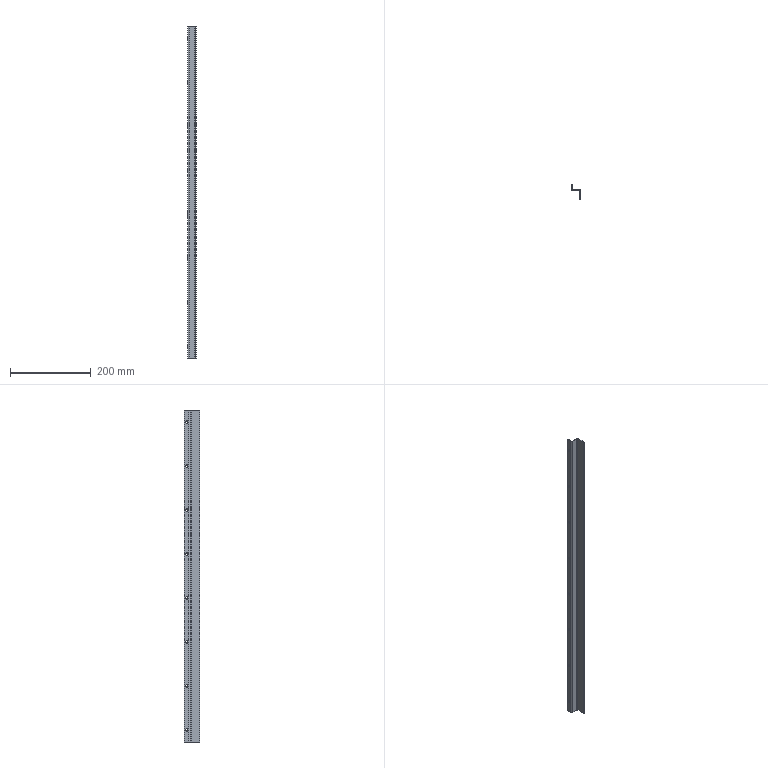Part | NX | features solid 2 | 1 solid | 30 faces | box 22 x 38 x 822 mm | volume 90666 mm3 | cylinder 20 | plane 10 | commonest cylinder face diameters 6 x16 4 x2 8 x2
STEP:
#1=CARTESIAN_POINT('',(-1106.,-748.,910.));
#2=VERTEX_POINT('',#1);
#3=CARTESIAN_POINT('',(-1108.,-748.,910.));
#4=VERTEX_POINT('',#3);
#5=CARTESIAN_POINT('',(-1929.172,-748.,910.));
#6=DIRECTION('',(1.,0.,0.));
#7=VECTOR('',#6,1000.);
#8=LINE('',#5,#7);
#9=EDGE_CURVE('',#2,#4,#8,.F.);
#10=ORIENTED_EDGE('',*,*,#9,.T.);
#11=CARTESIAN_POINT('',(-1108.,-742.,910.));
#12=VERTEX_POINT('',#11);
#13=CARTESIAN_POINT('',(-1108.,-745.,910.));
#14=DIRECTION('',(1.,0.,0.));
#15=DIRECTION('',(0.,1.,0.));
#16=AXIS2_PLACEMENT_3D('',#13,#14,#15);
#17=CIRCLE('',#16,3.);
#18=EDGE_CURVE('',#12,#4,#17,.T.);
#19=ORIENTED_EDGE('',*,*,#18,.F.);
#20=CARTESIAN_POINT('',(-1106.,-742.,910.));
#21=VERTEX_POINT('',#20);
#22=CARTESIAN_POINT('',(-1929.172,-742.,910.));
#23=DIRECTION('',(1.,0.,0.));
#24=VECTOR('',#23,1000.);
#25=LINE('',#22,#24);
#26=EDGE_CURVE('',#12,#21,#25,.T.);
#27=ORIENTED_EDGE('',*,*,#26,.T.);
#28=CARTESIAN_POINT('',(-1106.,-745.,910.));
#29=DIRECTION('',(1.,0.,0.));
#30=DIRECTION('',(0.,0.,-1.));
#31=AXIS2_PLACEMENT_3D('',#28,#29,#30);
#32=CIRCLE('',#31,3.);
#33=EDGE_CURVE('',#21,#2,#32,.T.);
#34=ORIENTED_EDGE('',*,*,#33,.T.);
#35=EDGE_LOOP('',(#10,#19,#27,#34));
#36=FACE_BOUND('',#35,.T.);
#37=CARTESIAN_POINT('',(-1929.172,-745.,910.));
#38=DIRECTION('',(1.,0.,0.));
#39=DIRECTION('',(0.,1.,0.));
#40=AXIS2_PLACEMENT_3D('',#37,#38,#39);
#41=CYLINDRICAL_SURFACE('',#40,3.);
#42=ADVANCED_FACE('',(#36),#41,.F.);
#43=CARTESIAN_POINT('',(-1088.,-756.,118.));
#44=VERTEX_POINT('',#43);
#45=CARTESIAN_POINT('',(-1088.,-777.,118.));
#46=VERTEX_POINT('',#45);
#47=CARTESIAN_POINT('',(-1088.,-754.,118.));
#48=DIRECTION('',(0.,-1.,0.));
#49=VECTOR('',#48,1000.);
#50=LINE('',#47,#49);
#51=EDGE_CURVE('',#44,#46,#50,.T.);
#52=ORIENTED_EDGE('',*,*,#51,.T.);
#53=CARTESIAN_POINT('',(-1088.,-777.,940.));
#54=VERTEX_POINT('',#53);
#55=CARTESIAN_POINT('',(-1088.,-777.,940.));
#56=DIRECTION('',(0.,0.,-1.));
#57=VECTOR('',#56,1000.);
#58=LINE('',#55,#57);
#59=EDGE_CURVE('',#54,#46,#58,.T.);
#60=ORIENTED_EDGE('',*,*,#59,.F.);
#61=CARTESIAN_POINT('',(-1088.,-756.,940.));
#62=VERTEX_POINT('',#61);
#63=CARTESIAN_POINT('',(-1088.,-754.,940.));
#64=DIRECTION('',(0.,-1.,0.));
#65=VECTOR('',#64,1000.);
#66=LINE('',#63,#65);
#67=EDGE_CURVE('',#62,#54,#66,.T.);
#68=ORIENTED_EDGE('',*,*,#67,.F.);
#69=CARTESIAN_POINT('',(-1088.,-756.,940.));
#70=DIRECTION('',(0.,0.,-1.));
#71=VECTOR('',#70,1000.);
#72=LINE('',#69,#71);
#73=EDGE_CURVE('',#62,#44,#72,.T.);
#74=ORIENTED_EDGE('',*,*,#73,.T.);
#75=EDGE_LOOP('',(#52,#60,#68,#74));
#76=FACE_BOUND('',#75,.T.);
#77=CARTESIAN_POINT('',(-1088.,-754.,940.));
#78=DIRECTION('',(1.,0.,0.));
#79=DIRECTION('',(0.,-1.,0.));
#80=AXIS2_PLACEMENT_3D('',#77,#78,#79);
#81=PLANE('',#80);
#82=ADVANCED_FACE('',(#76),#81,.F.);
#83=CARTESIAN_POINT('',(-1090.,-754.,118.));
#84=VERTEX_POINT('',#83);
#85=CARTESIAN_POINT('',(-1090.,-756.,118.));
#86=DIRECTION('',(0.,0.,-1.));
#87=DIRECTION('',(0.,1.,0.));
#88=AXIS2_PLACEMENT_3D('',#85,#86,#87);
#89=CIRCLE('',#88,2.);
#90=EDGE_CURVE('',#84,#44,#89,.T.);
#91=ORIENTED_EDGE('',*,*,#90,.T.);
#92=ORIENTED_EDGE('',*,*,#73,.F.);
#93=CARTESIAN_POINT('',(-1090.,-754.,940.));
#94=VERTEX_POINT('',#93);
#95=CARTESIAN_POINT('',(-1090.,-756.,940.));
#96=DIRECTION('',(0.,0.,-1.));
#97=DIRECTION('',(0.,1.,0.));
#98=AXIS2_PLACEMENT_3D('',#95,#96,#97);
#99=CIRCLE('',#98,2.);
#100=EDGE_CURVE('',#94,#62,#99,.T.);
#101=ORIENTED_EDGE('',*,*,#100,.F.);
#102=CARTESIAN_POINT('',(-1090.,-754.,940.));
#103=DIRECTION('',(0.,0.,-1.));
#104=VECTOR('',#103,1000.);
#105=LINE('',#102,#104);
#106=EDGE_CURVE('',#94,#84,#105,.T.);
#107=ORIENTED_EDGE('',*,*,#106,.T.);
#108=EDGE_LOOP('',(#91,#92,#101,#107));
#109=FACE_BOUND('',#108,.T.);
#110=CARTESIAN_POINT('',(-1090.,-756.,940.));
#111=DIRECTION('',(0.,0.,-1.));
#112=DIRECTION('',(0.,-1.,0.));
#113=AXIS2_PLACEMENT_3D('',#110,#111,#112);
#114=CYLINDRICAL_SURFACE('',#113,2.);
#115=ADVANCED_FACE('',(#109),#114,.F.);
#116=CARTESIAN_POINT('',(-1104.,-754.,118.));
#117=VERTEX_POINT('',#116);
#118=CARTESIAN_POINT('',(-1108.,-754.,118.));
#119=DIRECTION('',(1.,0.,0.));
#120=VECTOR('',#119,1000.);
#121=LINE('',#118,#120);
#122=EDGE_CURVE('',#117,#84,#121,.T.);
#123=ORIENTED_EDGE('',*,*,#122,.T.);
#124=ORIENTED_EDGE('',*,*,#106,.F.);
#125=CARTESIAN_POINT('',(-1104.,-754.,940.));
#126=VERTEX_POINT('',#125);
#127=CARTESIAN_POINT('',(-1108.,-754.,940.));
#128=DIRECTION('',(1.,0.,0.));
#129=VECTOR('',#128,1000.);
#130=LINE('',#127,#129);
#131=EDGE_CURVE('',#126,#94,#130,.T.);
#132=ORIENTED_EDGE('',*,*,#131,.F.);
#133=CARTESIAN_POINT('',(-1104.,-754.,940.));
#134=DIRECTION('',(0.,0.,-1.));
#135=VECTOR('',#134,1000.);
#136=LINE('',#133,#135);
#137=EDGE_CURVE('',#126,#117,#136,.T.);
#138=ORIENTED_EDGE('',*,*,#137,.T.);
#139=EDGE_LOOP('',(#123,#124,#132,#138));
#140=FACE_BOUND('',#139,.T.);
#141=CARTESIAN_POINT('',(-1108.,-754.,940.));
#142=DIRECTION('',(0.,1.,0.));
#143=DIRECTION('',(0.,0.,-1.));
#144=AXIS2_PLACEMENT_3D('',#141,#142,#143);
#145=PLANE('',#144);
#146=ADVANCED_FACE('',(#140),#145,.F.);
#147=CARTESIAN_POINT('',(-1108.,-750.,118.));
#148=VERTEX_POINT('',#147);
#149=CARTESIAN_POINT('',(-1104.,-750.,118.));
#150=DIRECTION('',(0.,0.,1.));
#151=DIRECTION('',(0.,-1.,0.));
#152=AXIS2_PLACEMENT_3D('',#149,#150,#151);
#153=CIRCLE('',#152,4.);
#154=EDGE_CURVE('',#148,#117,#153,.T.);
#155=ORIENTED_EDGE('',*,*,#154,.T.);
#156=ORIENTED_EDGE('',*,*,#137,.F.);
#157=CARTESIAN_POINT('',(-1108.,-750.,940.));
#158=VERTEX_POINT('',#157);
#159=CARTESIAN_POINT('',(-1104.,-750.,940.));
#160=DIRECTION('',(0.,0.,1.));
#161=DIRECTION('',(0.,-1.,0.));
#162=AXIS2_PLACEMENT_3D('',#159,#160,#161);
#163=CIRCLE('',#162,4.);
#164=EDGE_CURVE('',#158,#126,#163,.T.);
#165=ORIENTED_EDGE('',*,*,#164,.F.);
#166=CARTESIAN_POINT('',(-1108.,-750.,940.));
#167=DIRECTION('',(0.,0.,-1.));
#168=VECTOR('',#167,1000.);
#169=LINE('',#166,#168);
#170=EDGE_CURVE('',#158,#148,#169,.T.);
#171=ORIENTED_EDGE('',*,*,#170,.T.);
#172=EDGE_LOOP('',(#155,#156,#165,#171));
#173=FACE_BOUND('',#172,.T.);
#174=CARTESIAN_POINT('',(-1104.,-750.,940.));
#175=DIRECTION('',(0.,0.,-1.));
#176=DIRECTION('',(0.,-1.,0.));
#177=AXIS2_PLACEMENT_3D('',#174,#175,#176);
#178=CYLINDRICAL_SURFACE('',#177,4.);
#179=ADVANCED_FACE('',(#173),#178,.T.);
#180=ORIENTED_EDGE('',*,*,#18,.T.);
#181=CARTESIAN_POINT('',(-1108.,-745.,910.));
#182=DIRECTION('',(1.,0.,0.));
#183=DIRECTION('',(0.,1.,0.));
#184=AXIS2_PLACEMENT_3D('',#181,#182,#183);
#185=CIRCLE('',#184,3.);
#186=EDGE_CURVE('',#4,#12,#185,.T.);
#187=ORIENTED_EDGE('',*,*,#186,.T.);
#188=EDGE_LOOP('',(#180,#187));
#189=FACE_BOUND('',#188,.T.);
#190=CARTESIAN_POINT('',(-1108.,-742.,801.143));
#191=VERTEX_POINT('',#190);
#192=CARTESIAN_POINT('',(-1108.,-748.,801.143));
#193=VERTEX_POINT('',#192);
#194=CARTESIAN_POINT('',(-1108.,-745.,801.143));
#195=DIRECTION('',(1.,0.,0.));
#196=DIRECTION('',(0.,1.,0.));
#197=AXIS2_PLACEMENT_3D('',#194,#195,#196);
#198=CIRCLE('',#197,3.);
#199=EDGE_CURVE('',#191,#193,#198,.T.);
#200=ORIENTED_EDGE('',*,*,#199,.T.);
#201=CARTESIAN_POINT('',(-1108.,-745.,801.143));
#202=DIRECTION('',(1.,0.,0.));
#203=DIRECTION('',(0.,1.,0.));
#204=AXIS2_PLACEMENT_3D('',#201,#202,#203);
#205=CIRCLE('',#204,3.);
#206=EDGE_CURVE('',#193,#191,#205,.T.);
#207=ORIENTED_EDGE('',*,*,#206,.T.);
#208=EDGE_LOOP('',(#200,#207));
#209=FACE_BOUND('',#208,.T.);
#210=CARTESIAN_POINT('',(-1108.,-742.,692.286));
#211=VERTEX_POINT('',#210);
#212=CARTESIAN_POINT('',(-1108.,-748.,692.286));
#213=VERTEX_POINT('',#212);
#214=CARTESIAN_POINT('',(-1108.,-745.,692.286));
#215=DIRECTION('',(1.,0.,0.));
#216=DIRECTION('',(0.,1.,0.));
#217=AXIS2_PLACEMENT_3D('',#214,#215,#216);
#218=CIRCLE('',#217,3.);
#219=EDGE_CURVE('',#211,#213,#218,.T.);
#220=ORIENTED_EDGE('',*,*,#219,.T.);
#221=CARTESIAN_POINT('',(-1108.,-745.,692.286));
#222=DIRECTION('',(1.,0.,0.));
#223=DIRECTION('',(0.,1.,0.));
#224=AXIS2_PLACEMENT_3D('',#221,#222,#223);
#225=CIRCLE('',#224,3.);
#226=EDGE_CURVE('',#213,#211,#225,.T.);
#227=ORIENTED_EDGE('',*,*,#226,.T.);
#228=EDGE_LOOP('',(#220,#227));
#229=FACE_BOUND('',#228,.T.);
#230=CARTESIAN_POINT('',(-1108.,-742.,583.429));
#231=VERTEX_POINT('',#230);
#232=CARTESIAN_POINT('',(-1108.,-748.,583.429));
#233=VERTEX_POINT('',#232);
#234=CARTESIAN_POINT('',(-1108.,-745.,583.429));
#235=DIRECTION('',(1.,0.,0.));
#236=DIRECTION('',(0.,1.,0.));
#237=AXIS2_PLACEMENT_3D('',#234,#235,#236);
#238=CIRCLE('',#237,3.);
#239=EDGE_CURVE('',#231,#233,#238,.T.);
#240=ORIENTED_EDGE('',*,*,#239,.T.);
#241=CARTESIAN_POINT('',(-1108.,-745.,583.429));
#242=DIRECTION('',(1.,0.,0.));
#243=DIRECTION('',(0.,1.,0.));
#244=AXIS2_PLACEMENT_3D('',#241,#242,#243);
#245=CIRCLE('',#244,3.);
#246=EDGE_CURVE('',#233,#231,#245,.T.);
#247=ORIENTED_EDGE('',*,*,#246,.T.);
#248=EDGE_LOOP('',(#240,#247));
#249=FACE_BOUND('',#248,.T.);
#250=CARTESIAN_POINT('',(-1108.,-742.,474.571));
#251=VERTEX_POINT('',#250);
#252=CARTESIAN_POINT('',(-1108.,-748.,474.571));
#253=VERTEX_POINT('',#252);
#254=CARTESIAN_POINT('',(-1108.,-745.,474.571));
#255=DIRECTION('',(1.,0.,0.));
#256=DIRECTION('',(0.,1.,0.));
#257=AXIS2_PLACEMENT_3D('',#254,#255,#256);
#258=CIRCLE('',#257,3.);
#259=EDGE_CURVE('',#251,#253,#258,.T.);
#260=ORIENTED_EDGE('',*,*,#259,.T.);
#261=CARTESIAN_POINT('',(-1108.,-745.,474.571));
#262=DIRECTION('',(1.,0.,0.));
#263=DIRECTION('',(0.,1.,0.));
#264=AXIS2_PLACEMENT_3D('',#261,#262,#263);
#265=CIRCLE('',#264,3.);
#266=EDGE_CURVE('',#253,#251,#265,.T.);
#267=ORIENTED_EDGE('',*,*,#266,.T.);
#268=EDGE_LOOP('',(#260,#267));
#269=FACE_BOUND('',#268,.T.);
#270=CARTESIAN_POINT('',(-1108.,-742.,365.714));
#271=VERTEX_POINT('',#270);
#272=CARTESIAN_POINT('',(-1108.,-748.,365.714));
#273=VERTEX_POINT('',#272);
#274=CARTESIAN_POINT('',(-1108.,-745.,365.714));
#275=DIRECTION('',(1.,0.,0.));
#276=DIRECTION('',(0.,1.,0.));
#277=AXIS2_PLACEMENT_3D('',#274,#275,#276);
#278=CIRCLE('',#277,3.);
#279=EDGE_CURVE('',#271,#273,#278,.T.);
#280=ORIENTED_EDGE('',*,*,#279,.T.);
#281=CARTESIAN_POINT('',(-1108.,-745.,365.714));
#282=DIRECTION('',(1.,0.,0.));
#283=DIRECTION('',(0.,1.,0.));
#284=AXIS2_PLACEMENT_3D('',#281,#282,#283);
#285=CIRCLE('',#284,3.);
#286=EDGE_CURVE('',#273,#271,#285,.T.);
#287=ORIENTED_EDGE('',*,*,#286,.T.);
#288=EDGE_LOOP('',(#280,#287));
#289=FACE_BOUND('',#288,.T.);
#290=CARTESIAN_POINT('',(-1108.,-742.,256.857));
#291=VERTEX_POINT('',#290);
#292=CARTESIAN_POINT('',(-1108.,-748.,256.857));
#293=VERTEX_POINT('',#292);
#294=CARTESIAN_POINT('',(-1108.,-745.,256.857));
#295=DIRECTION('',(1.,0.,0.));
#296=DIRECTION('',(0.,1.,0.));
#297=AXIS2_PLACEMENT_3D('',#294,#295,#296);
#298=CIRCLE('',#297,3.);
#299=EDGE_CURVE('',#291,#293,#298,.T.);
#300=ORIENTED_EDGE('',*,*,#299,.T.);
#301=CARTESIAN_POINT('',(-1108.,-745.,256.857));
#302=DIRECTION('',(1.,0.,0.));
#303=DIRECTION('',(0.,1.,0.));
#304=AXIS2_PLACEMENT_3D('',#301,#302,#303);
#305=CIRCLE('',#304,3.);
#306=EDGE_CURVE('',#293,#291,#305,.T.);
#307=ORIENTED_EDGE('',*,*,#306,.T.);
#308=EDGE_LOOP('',(#300,#307));
#309=FACE_BOUND('',#308,.T.);
#310=CARTESIAN_POINT('',(-1108.,-742.,148.));
#311=VERTEX_POINT('',#310);
#312=CARTESIAN_POINT('',(-1108.,-748.,148.));
#313=VERTEX_POINT('',#312);
#314=CARTESIAN_POINT('',(-1108.,-745.,148.));
#315=DIRECTION('',(1.,0.,0.));
#316=DIRECTION('',(0.,1.,0.));
#317=AXIS2_PLACEMENT_3D('',#314,#315,#316);
#318=CIRCLE('',#317,3.);
#319=EDGE_CURVE('',#311,#313,#318,.T.);
#320=ORIENTED_EDGE('',*,*,#319,.T.);
#321=CARTESIAN_POINT('',(-1108.,-745.,148.));
#322=DIRECTION('',(1.,0.,0.));
#323=DIRECTION('',(0.,1.,0.));
#324=AXIS2_PLACEMENT_3D('',#321,#322,#323);
#325=CIRCLE('',#324,3.);
#326=EDGE_CURVE('',#313,#311,#325,.T.);
#327=ORIENTED_EDGE('',*,*,#326,.T.);
#328=EDGE_LOOP('',(#320,#327));
#329=FACE_BOUND('',#328,.T.);
#330=CARTESIAN_POINT('',(-1108.,-739.,118.));
#331=VERTEX_POINT('',#330);
#332=CARTESIAN_POINT('',(-1108.,-739.,118.));
#333=DIRECTION('',(0.,-1.,0.));
#334=VECTOR('',#333,1000.);
#335=LINE('',#332,#334);
#336=EDGE_CURVE('',#331,#148,#335,.T.);
#337=ORIENTED_EDGE('',*,*,#336,.T.);
#338=ORIENTED_EDGE('',*,*,#170,.F.);
#339=CARTESIAN_POINT('',(-1108.,-739.,940.));
#340=VERTEX_POINT('',#339);
#341=CARTESIAN_POINT('',(-1108.,-739.,940.));
#342=DIRECTION('',(0.,-1.,0.));
#343=VECTOR('',#342,1000.);
#344=LINE('',#341,#343);
#345=EDGE_CURVE('',#340,#158,#344,.T.);
#346=ORIENTED_EDGE('',*,*,#345,.F.);
#347=CARTESIAN_POINT('',(-1108.,-739.,940.));
#348=DIRECTION('',(0.,0.,-1.));
#349=VECTOR('',#348,1000.);
#350=LINE('',#347,#349);
#351=EDGE_CURVE('',#340,#331,#350,.T.);
#352=ORIENTED_EDGE('',*,*,#351,.T.);
#353=EDGE_LOOP('',(#337,#338,#346,#352));
#354=FACE_BOUND('',#353,.T.);
#355=CARTESIAN_POINT('',(-1108.,-739.,940.));
#356=DIRECTION('',(1.,0.,0.));
#357=DIRECTION('',(0.,-1.,0.));
#358=AXIS2_PLACEMENT_3D('',#355,#356,#357);
#359=PLANE('',#358);
#360=ADVANCED_FACE('',(#189,#209,#229,#249,#269,#289,#309,#329,#354),#359,.F.);
#361=CARTESIAN_POINT('',(-1086.,-756.,118.));
#362=VERTEX_POINT('',#361);
#363=CARTESIAN_POINT('',(-1086.,-777.,118.));
#364=VERTEX_POINT('',#363);
#365=CARTESIAN_POINT('',(-1086.,-754.,118.));
#366=DIRECTION('',(0.,-1.,0.));
#367=VECTOR('',#366,1000.);
#368=LINE('',#365,#367);
#369=EDGE_CURVE('',#362,#364,#368,.T.);
#370=ORIENTED_EDGE('',*,*,#369,.F.);
#371=CARTESIAN_POINT('',(-1086.,-756.,940.));
#372=VERTEX_POINT('',#371);
#373=CARTESIAN_POINT('',(-1086.,-756.,940.));
#374=DIRECTION('',(0.,0.,-1.));
#375=VECTOR('',#374,1000.);
#376=LINE('',#373,#375);
#377=EDGE_CURVE('',#372,#362,#376,.T.);
#378=ORIENTED_EDGE('',*,*,#377,.F.);
#379=CARTESIAN_POINT('',(-1086.,-777.,940.));
#380=VERTEX_POINT('',#379);
#381=CARTESIAN_POINT('',(-1086.,-754.,940.));
#382=DIRECTION('',(0.,-1.,0.));
#383=VECTOR('',#382,1000.);
#384=LINE('',#381,#383);
#385=EDGE_CURVE('',#372,#380,#384,.T.);
#386=ORIENTED_EDGE('',*,*,#385,.T.);
#387=CARTESIAN_POINT('',(-1086.,-777.,940.));
#388=DIRECTION('',(0.,0.,-1.));
#389=VECTOR('',#388,1000.);
#390=LINE('',#387,#389);
#391=EDGE_CURVE('',#380,#364,#390,.T.);
#392=ORIENTED_EDGE('',*,*,#391,.T.);
#393=EDGE_LOOP('',(#370,#378,#386,#392));
#394=FACE_BOUND('',#393,.T.);
#395=CARTESIAN_POINT('',(-1086.,-754.,940.));
#396=DIRECTION('',(1.,0.,0.));
#397=DIRECTION('',(0.,-1.,0.));
#398=AXIS2_PLACEMENT_3D('',#395,#396,#397);
#399=PLANE('',#398);
#400=ADVANCED_FACE('',(#394),#399,.T.);
#401=CARTESIAN_POINT('',(-1090.,-752.,118.));
#402=VERTEX_POINT('',#401);
#403=CARTESIAN_POINT('',(-1090.,-756.,118.));
#404=DIRECTION('',(0.,0.,-1.));
#405=DIRECTION('',(0.,-1.,0.));
#406=AXIS2_PLACEMENT_3D('',#403,#404,#405);
#407=CIRCLE('',#406,4.);
#408=EDGE_CURVE('',#402,#362,#407,.T.);
#409=ORIENTED_EDGE('',*,*,#408,.F.);
#410=CARTESIAN_POINT('',(-1090.,-752.,940.));
#411=VERTEX_POINT('',#410);
#412=CARTESIAN_POINT('',(-1090.,-752.,940.));
#413=DIRECTION('',(0.,0.,-1.));
#414=VECTOR('',#413,1000.);
#415=LINE('',#412,#414);
#416=EDGE_CURVE('',#411,#402,#415,.T.);
#417=ORIENTED_EDGE('',*,*,#416,.F.);
#418=CARTESIAN_POINT('',(-1090.,-756.,940.));
#419=DIRECTION('',(0.,0.,-1.));
#420=DIRECTION('',(0.,-1.,0.));
#421=AXIS2_PLACEMENT_3D('',#418,#419,#420);
#422=CIRCLE('',#421,4.);
#423=EDGE_CURVE('',#411,#372,#422,.T.);
#424=ORIENTED_EDGE('',*,*,#423,.T.);
#425=ORIENTED_EDGE('',*,*,#377,.T.);
#426=EDGE_LOOP('',(#409,#417,#424,#425));
#427=FACE_BOUND('',#426,.T.);
#428=CARTESIAN_POINT('',(-1090.,-756.,940.));
#429=DIRECTION('',(0.,0.,-1.));
#430=DIRECTION('',(0.,-1.,0.));
#431=AXIS2_PLACEMENT_3D('',#428,#429,#430);
#432=CYLINDRICAL_SURFACE('',#431,4.);
#433=ADVANCED_FACE('',(#427),#432,.T.);
#434=CARTESIAN_POINT('',(-1104.,-752.,118.));
#435=VERTEX_POINT('',#434);
#436=CARTESIAN_POINT('',(-1108.,-752.,118.));
#437=DIRECTION('',(1.,0.,0.));
#438=VECTOR('',#437,1000.);
#439=LINE('',#436,#438);
#440=EDGE_CURVE('',#435,#402,#439,.T.);
#441=ORIENTED_EDGE('',*,*,#440,.F.);
#442=CARTESIAN_POINT('',(-1104.,-752.,940.));
#443=VERTEX_POINT('',#442);
#444=CARTESIAN_POINT('',(-1104.,-752.,940.));
#445=DIRECTION('',(0.,0.,-1.));
#446=VECTOR('',#445,1000.);
#447=LINE('',#444,#446);
#448=EDGE_CURVE('',#443,#435,#447,.T.);
#449=ORIENTED_EDGE('',*,*,#448,.F.);
#450=CARTESIAN_POINT('',(-1108.,-752.,940.));
#451=DIRECTION('',(1.,0.,0.));
#452=VECTOR('',#451,1000.);
#453=LINE('',#450,#452);
#454=EDGE_CURVE('',#443,#411,#453,.T.);
#455=ORIENTED_EDGE('',*,*,#454,.T.);
#456=ORIENTED_EDGE('',*,*,#416,.T.);
#457=EDGE_LOOP('',(#441,#449,#455,#456));
#458=FACE_BOUND('',#457,.T.);
#459=CARTESIAN_POINT('',(-1108.,-752.,940.));
#460=DIRECTION('',(0.,1.,0.));
#461=DIRECTION('',(0.,0.,-1.));
#462=AXIS2_PLACEMENT_3D('',#459,#460,#461);
#463=PLANE('',#462);
#464=ADVANCED_FACE('',(#458),#463,.T.);
#465=CARTESIAN_POINT('',(-1106.,-750.,118.));
#466=VERTEX_POINT('',#465);
#467=CARTESIAN_POINT('',(-1104.,-750.,118.));
#468=DIRECTION('',(0.,0.,1.));
#469=DIRECTION('',(0.,-1.,0.));
#470=AXIS2_PLACEMENT_3D('',#467,#468,#469);
#471=CIRCLE('',#470,2.);
#472=EDGE_CURVE('',#466,#435,#471,.T.);
#473=ORIENTED_EDGE('',*,*,#472,.F.);
#474=CARTESIAN_POINT('',(-1106.,-750.,940.));
#475=VERTEX_POINT('',#474);
#476=CARTESIAN_POINT('',(-1106.,-750.,940.));
#477=DIRECTION('',(0.,0.,-1.));
#478=VECTOR('',#477,1000.);
#479=LINE('',#476,#478);
#480=EDGE_CURVE('',#475,#466,#479,.T.);
#481=ORIENTED_EDGE('',*,*,#480,.F.);
#482=CARTESIAN_POINT('',(-1104.,-750.,940.));
#483=DIRECTION('',(0.,0.,1.));
#484=DIRECTION('',(0.,-1.,0.));
#485=AXIS2_PLACEMENT_3D('',#482,#483,#484);
#486=CIRCLE('',#485,2.);
#487=EDGE_CURVE('',#475,#443,#486,.T.);
#488=ORIENTED_EDGE('',*,*,#487,.T.);
#489=ORIENTED_EDGE('',*,*,#448,.T.);
#490=EDGE_LOOP('',(#473,#481,#488,#489));
#491=FACE_BOUND('',#490,.T.);
#492=CARTESIAN_POINT('',(-1104.,-750.,940.));
#493=DIRECTION('',(0.,0.,-1.));
#494=DIRECTION('',(0.,-1.,0.));
#495=AXIS2_PLACEMENT_3D('',#492,#493,#494);
#496=CYLINDRICAL_SURFACE('',#495,2.);
#497=ADVANCED_FACE('',(#491),#496,.F.);
#498=ORIENTED_EDGE('',*,*,#33,.F.);
#499=CARTESIAN_POINT('',(-1106.,-745.,910.));
#500=DIRECTION('',(1.,0.,0.));
#501=DIRECTION('',(0.,0.,-1.));
#502=AXIS2_PLACEMENT_3D('',#499,#500,#501);
#503=CIRCLE('',#502,3.);
#504=EDGE_CURVE('',#2,#21,#503,.T.);
#505=ORIENTED_EDGE('',*,*,#504,.F.);
#506=EDGE_LOOP('',(#498,#505));
#507=FACE_BOUND('',#506,.T.);
#508=CARTESIAN_POINT('',(-1106.,-742.,801.143));
#509=VERTEX_POINT('',#508);
#510=CARTESIAN_POINT('',(-1106.,-748.,801.143));
#511=VERTEX_POINT('',#510);
#512=CARTESIAN_POINT('',(-1106.,-745.,801.143));
#513=DIRECTION('',(1.,0.,0.));
#514=DIRECTION('',(0.,0.,-1.));
#515=AXIS2_PLACEMENT_3D('',#512,#513,#514);
#516=CIRCLE('',#515,3.);
#517=EDGE_CURVE('',#509,#511,#516,.T.);
#518=ORIENTED_EDGE('',*,*,#517,.F.);
#519=CARTESIAN_POINT('',(-1106.,-745.,801.143));
#520=DIRECTION('',(1.,0.,0.));
#521=DIRECTION('',(0.,0.,-1.));
#522=AXIS2_PLACEMENT_3D('',#519,#520,#521);
#523=CIRCLE('',#522,3.);
#524=EDGE_CURVE('',#511,#509,#523,.T.);
#525=ORIENTED_EDGE('',*,*,#524,.F.);
#526=EDGE_LOOP('',(#518,#525));
#527=FACE_BOUND('',#526,.T.);
#528=CARTESIAN_POINT('',(-1106.,-742.,692.286));
#529=VERTEX_POINT('',#528);
#530=CARTESIAN_POINT('',(-1106.,-748.,692.286));
#531=VERTEX_POINT('',#530);
#532=CARTESIAN_POINT('',(-1106.,-745.,692.286));
#533=DIRECTION('',(1.,0.,0.));
#534=DIRECTION('',(0.,0.,-1.));
#535=AXIS2_PLACEMENT_3D('',#532,#533,#534);
#536=CIRCLE('',#535,3.);
#537=EDGE_CURVE('',#529,#531,#536,.T.);
#538=ORIENTED_EDGE('',*,*,#537,.F.);
#539=CARTESIAN_POINT('',(-1106.,-745.,692.286));
#540=DIRECTION('',(1.,0.,0.));
#541=DIRECTION('',(0.,0.,-1.));
#542=AXIS2_PLACEMENT_3D('',#539,#540,#541);
#543=CIRCLE('',#542,3.);
#544=EDGE_CURVE('',#531,#529,#543,.T.);
#545=ORIENTED_EDGE('',*,*,#544,.F.);
#546=EDGE_LOOP('',(#538,#545));
#547=FACE_BOUND('',#546,.T.);
#548=CARTESIAN_POINT('',(-1106.,-742.,583.429));
#549=VERTEX_POINT('',#548);
#550=CARTESIAN_POINT('',(-1106.,-748.,583.429));
#551=VERTEX_POINT('',#550);
#552=CARTESIAN_POINT('',(-1106.,-745.,583.429));
#553=DIRECTION('',(1.,0.,0.));
#554=DIRECTION('',(0.,0.,-1.));
#555=AXIS2_PLACEMENT_3D('',#552,#553,#554);
#556=CIRCLE('',#555,3.);
#557=EDGE_CURVE('',#549,#551,#556,.T.);
#558=ORIENTED_EDGE('',*,*,#557,.F.);
#559=CARTESIAN_POINT('',(-1106.,-745.,583.429));
#560=DIRECTION('',(1.,0.,0.));
#561=DIRECTION('',(0.,0.,-1.));
#562=AXIS2_PLACEMENT_3D('',#559,#560,#561);
#563=CIRCLE('',#562,3.);
#564=EDGE_CURVE('',#551,#549,#563,.T.);
#565=ORIENTED_EDGE('',*,*,#564,.F.);
#566=EDGE_LOOP('',(#558,#565));
#567=FACE_BOUND('',#566,.T.);
#568=CARTESIAN_POINT('',(-1106.,-742.,474.571));
#569=VERTEX_POINT('',#568);
#570=CARTESIAN_POINT('',(-1106.,-748.,474.571));
#571=VERTEX_POINT('',#570);
#572=CARTESIAN_POINT('',(-1106.,-745.,474.571));
#573=DIRECTION('',(1.,0.,0.));
#574=DIRECTION('',(0.,0.,-1.));
#575=AXIS2_PLACEMENT_3D('',#572,#573,#574);
#576=CIRCLE('',#575,3.);
#577=EDGE_CURVE('',#569,#571,#576,.T.);
#578=ORIENTED_EDGE('',*,*,#577,.F.);
#579=CARTESIAN_POINT('',(-1106.,-745.,474.571));
#580=DIRECTION('',(1.,0.,0.));
#581=DIRECTION('',(0.,0.,-1.));
#582=AXIS2_PLACEMENT_3D('',#579,#580,#581);
#583=CIRCLE('',#582,3.);
#584=EDGE_CURVE('',#571,#569,#583,.T.);
#585=ORIENTED_EDGE('',*,*,#584,.F.);
#586=EDGE_LOOP('',(#578,#585));
#587=FACE_BOUND('',#586,.T.);
#588=CARTESIAN_POINT('',(-1106.,-742.,365.714));
#589=VERTEX_POINT('',#588);
#590=CARTESIAN_POINT('',(-1106.,-748.,365.714));
#591=VERTEX_POINT('',#590);
#592=CARTESIAN_POINT('',(-1106.,-745.,365.714));
#593=DIRECTION('',(1.,0.,0.));
#594=DIRECTION('',(0.,0.,-1.));
#595=AXIS2_PLACEMENT_3D('',#592,#593,#594);
#596=CIRCLE('',#595,3.);
#597=EDGE_CURVE('',#589,#591,#596,.T.);
#598=ORIENTED_EDGE('',*,*,#597,.F.);
#599=CARTESIAN_POINT('',(-1106.,-745.,365.714));
#600=DIRECTION('',(1.,0.,0.));
#601=DIRECTION('',(0.,0.,-1.));
#602=AXIS2_PLACEMENT_3D('',#599,#600,#601);
#603=CIRCLE('',#602,3.);
#604=EDGE_CURVE('',#591,#589,#603,.T.);
#605=ORIENTED_EDGE('',*,*,#604,.F.);
#606=EDGE_LOOP('',(#598,#605));
#607=FACE_BOUND('',#606,.T.);
#608=CARTESIAN_POINT('',(-1106.,-742.,256.857));
#609=VERTEX_POINT('',#608);
#610=CARTESIAN_POINT('',(-1106.,-748.,256.857));
#611=VERTEX_POINT('',#610);
#612=CARTESIAN_POINT('',(-1106.,-745.,256.857));
#613=DIRECTION('',(1.,0.,0.));
#614=DIRECTION('',(0.,0.,-1.));
#615=AXIS2_PLACEMENT_3D('',#612,#613,#614);
#616=CIRCLE('',#615,3.);
#617=EDGE_CURVE('',#609,#611,#616,.T.);
#618=ORIENTED_EDGE('',*,*,#617,.F.);
#619=CARTESIAN_POINT('',(-1106.,-745.,256.857));
#620=DIRECTION('',(1.,0.,0.));
#621=DIRECTION('',(0.,0.,-1.));
#622=AXIS2_PLACEMENT_3D('',#619,#620,#621);
#623=CIRCLE('',#622,3.);
#624=EDGE_CURVE('',#611,#609,#623,.T.);
#625=ORIENTED_EDGE('',*,*,#624,.F.);
#626=EDGE_LOOP('',(#618,#625));
#627=FACE_BOUND('',#626,.T.);
#628=CARTESIAN_POINT('',(-1106.,-742.,148.));
#629=VERTEX_POINT('',#628);
#630=CARTESIAN_POINT('',(-1106.,-748.,148.));
#631=VERTEX_POINT('',#630);
#632=CARTESIAN_POINT('',(-1106.,-745.,148.));
#633=DIRECTION('',(1.,0.,0.));
#634=DIRECTION('',(0.,0.,-1.));
#635=AXIS2_PLACEMENT_3D('',#632,#633,#634);
#636=CIRCLE('',#635,3.);
#637=EDGE_CURVE('',#629,#631,#636,.T.);
#638=ORIENTED_EDGE('',*,*,#637,.F.);
#639=CARTESIAN_POINT('',(-1106.,-745.,148.));
#640=DIRECTION('',(1.,0.,0.));
#641=DIRECTION('',(0.,0.,-1.));
#642=AXIS2_PLACEMENT_3D('',#639,#640,#641);
#643=CIRCLE('',#642,3.);
#644=EDGE_CURVE('',#631,#629,#643,.T.);
#645=ORIENTED_EDGE('',*,*,#644,.F.);
#646=EDGE_LOOP('',(#638,#645));
#647=FACE_BOUND('',#646,.T.);
#648=CARTESIAN_POINT('',(-1106.,-739.,118.));
#649=VERTEX_POINT('',#648);
#650=CARTESIAN_POINT('',(-1106.,-739.,118.));
#651=DIRECTION('',(0.,-1.,0.));
#652=VECTOR('',#651,1000.);
#653=LINE('',#650,#652);
#654=EDGE_CURVE('',#649,#466,#653,.T.);
#655=ORIENTED_EDGE('',*,*,#654,.F.);
#656=CARTESIAN_POINT('',(-1106.,-739.,940.));
#657=VERTEX_POINT('',#656);
#658=CARTESIAN_POINT('',(-1106.,-739.,940.));
#659=DIRECTION('',(0.,0.,-1.));
#660=VECTOR('',#659,1000.);
#661=LINE('',#658,#660);
#662=EDGE_CURVE('',#657,#649,#661,.T.);
#663=ORIENTED_EDGE('',*,*,#662,.F.);
#664=CARTESIAN_POINT('',(-1106.,-739.,940.));
#665=DIRECTION('',(0.,-1.,0.));
#666=VECTOR('',#665,1000.);
#667=LINE('',#664,#666);
#668=EDGE_CURVE('',#657,#475,#667,.T.);
#669=ORIENTED_EDGE('',*,*,#668,.T.);
#670=ORIENTED_EDGE('',*,*,#480,.T.);
#671=EDGE_LOOP('',(#655,#663,#669,#670));
#672=FACE_BOUND('',#671,.T.);
#673=CARTESIAN_POINT('',(-1106.,-739.,940.));
#674=DIRECTION('',(1.,0.,0.));
#675=DIRECTION('',(0.,-1.,0.));
#676=AXIS2_PLACEMENT_3D('',#673,#674,#675);
#677=PLANE('',#676);
#678=ADVANCED_FACE('',(#507,#527,#547,#567,#587,#607,#627,#647,#672),#677,.T.);
#679=ORIENTED_EDGE('',*,*,#351,.F.);
#680=CARTESIAN_POINT('',(-1108.,-739.,940.));
#681=DIRECTION('',(1.,0.,0.));
#682=VECTOR('',#681,1000.);
#683=LINE('',#680,#682);
#684=EDGE_CURVE('',#340,#657,#683,.T.);
#685=ORIENTED_EDGE('',*,*,#684,.T.);
#686=ORIENTED_EDGE('',*,*,#662,.T.);
#687=CARTESIAN_POINT('',(-1108.,-739.,118.));
#688=DIRECTION('',(1.,0.,0.));
#689=VECTOR('',#688,1000.);
#690=LINE('',#687,#689);
#691=EDGE_CURVE('',#331,#649,#690,.T.);
#692=ORIENTED_EDGE('',*,*,#691,.F.);
#693=EDGE_LOOP('',(#679,#685,#686,#692));
#694=FACE_BOUND('',#693,.T.);
#695=CARTESIAN_POINT('',(-1108.,-739.,940.));
#696=DIRECTION('',(0.,-1.,0.));
#697=DIRECTION('',(-1.,0.,0.));
#698=AXIS2_PLACEMENT_3D('',#695,#696,#697);
#699=PLANE('',#698);
#700=ADVANCED_FACE('',(#694),#699,.F.);
#701=ORIENTED_EDGE('',*,*,#654,.T.);
#702=ORIENTED_EDGE('',*,*,#472,.T.);
#703=ORIENTED_EDGE('',*,*,#440,.T.);
#704=ORIENTED_EDGE('',*,*,#408,.T.);
#705=ORIENTED_EDGE('',*,*,#369,.T.);
#706=CARTESIAN_POINT('',(-1088.,-777.,118.));
#707=DIRECTION('',(1.,0.,0.));
#708=VECTOR('',#707,1000.);
#709=LINE('',#706,#708);
#710=EDGE_CURVE('',#46,#364,#709,.T.);
#711=ORIENTED_EDGE('',*,*,#710,.F.);
#712=ORIENTED_EDGE('',*,*,#51,.F.);
#713=ORIENTED_EDGE('',*,*,#90,.F.);
#714=ORIENTED_EDGE('',*,*,#122,.F.);
#715=ORIENTED_EDGE('',*,*,#154,.F.);
#716=ORIENTED_EDGE('',*,*,#336,.F.);
#717=ORIENTED_EDGE('',*,*,#691,.T.);
#718=EDGE_LOOP('',(#701,#702,#703,#704,#705,#711,#712,#713,#714,#715,#716,#717));
#719=FACE_BOUND('',#718,.T.);
#720=CARTESIAN_POINT('',(-1108.,-739.,118.));
#721=DIRECTION('',(0.,0.,1.));
#722=DIRECTION('',(0.,-1.,0.));
#723=AXIS2_PLACEMENT_3D('',#720,#721,#722);
#724=PLANE('',#723);
#725=ADVANCED_FACE('',(#719),#724,.F.);
#726=CARTESIAN_POINT('',(-1088.,-777.,940.));
#727=DIRECTION('',(1.,0.,0.));
#728=VECTOR('',#727,1000.);
#729=LINE('',#726,#728);
#730=EDGE_CURVE('',#54,#380,#729,.T.);
#731=ORIENTED_EDGE('',*,*,#730,.F.);
#732=ORIENTED_EDGE('',*,*,#59,.T.);
#733=ORIENTED_EDGE('',*,*,#710,.T.);
#734=ORIENTED_EDGE('',*,*,#391,.F.);
#735=EDGE_LOOP('',(#731,#732,#733,#734));
#736=FACE_BOUND('',#735,.T.);
#737=CARTESIAN_POINT('',(-1088.,-777.,940.));
#738=DIRECTION('',(0.,-1.,0.));
#739=DIRECTION('',(-1.,0.,0.));
#740=AXIS2_PLACEMENT_3D('',#737,#738,#739);
#741=PLANE('',#740);
#742=ADVANCED_FACE('',(#736),#741,.T.);
#743=ORIENTED_EDGE('',*,*,#385,.F.);
#744=ORIENTED_EDGE('',*,*,#423,.F.);
#745=ORIENTED_EDGE('',*,*,#454,.F.);
#746=ORIENTED_EDGE('',*,*,#487,.F.);
#747=ORIENTED_EDGE('',*,*,#668,.F.);
#748=ORIENTED_EDGE('',*,*,#684,.F.);
#749=ORIENTED_EDGE('',*,*,#345,.T.);
#750=ORIENTED_EDGE('',*,*,#164,.T.);
#751=ORIENTED_EDGE('',*,*,#131,.T.);
#752=ORIENTED_EDGE('',*,*,#100,.T.);
#753=ORIENTED_EDGE('',*,*,#67,.T.);
#754=ORIENTED_EDGE('',*,*,#730,.T.);
#755=EDGE_LOOP('',(#743,#744,#745,#746,#747,#748,#749,#750,#751,#752,#753,#754));
#756=FACE_BOUND('',#755,.T.);
#757=CARTESIAN_POINT('',(-1088.,-754.,940.));
#758=DIRECTION('',(0.,0.,1.));
#759=DIRECTION('',(0.,-1.,0.));
#760=AXIS2_PLACEMENT_3D('',#757,#758,#759);
#761=PLANE('',#760);
#762=ADVANCED_FACE('',(#756),#761,.T.);
#763=CARTESIAN_POINT('',(-1929.172,-748.,801.143));
#764=DIRECTION('',(1.,0.,0.));
#765=VECTOR('',#764,1000.);
#766=LINE('',#763,#765);
#767=EDGE_CURVE('',#193,#511,#766,.T.);
#768=ORIENTED_EDGE('',*,*,#767,.F.);
#769=ORIENTED_EDGE('',*,*,#199,.F.);
#770=CARTESIAN_POINT('',(-1929.172,-742.,801.143));
#771=DIRECTION('',(1.,0.,0.));
#772=VECTOR('',#771,1000.);
#773=LINE('',#770,#772);
#774=EDGE_CURVE('',#509,#191,#773,.F.);
#775=ORIENTED_EDGE('',*,*,#774,.F.);
#776=ORIENTED_EDGE('',*,*,#517,.T.);
#777=EDGE_LOOP('',(#768,#769,#775,#776));
#778=FACE_BOUND('',#777,.T.);
#779=CARTESIAN_POINT('',(-1929.172,-745.,801.143));
#780=DIRECTION('',(1.,0.,0.));
#781=DIRECTION('',(0.,1.,0.));
#782=AXIS2_PLACEMENT_3D('',#779,#780,#781);
#783=CYLINDRICAL_SURFACE('',#782,3.);
#784=ADVANCED_FACE('',(#778),#783,.F.);
#785=CARTESIAN_POINT('',(-1929.172,-748.,692.286));
#786=DIRECTION('',(1.,0.,0.));
#787=VECTOR('',#786,1000.);
#788=LINE('',#785,#787);
#789=EDGE_CURVE('',#213,#531,#788,.T.);
#790=ORIENTED_EDGE('',*,*,#789,.F.);
#791=ORIENTED_EDGE('',*,*,#219,.F.);
#792=CARTESIAN_POINT('',(-1929.172,-742.,692.286));
#793=DIRECTION('',(1.,0.,0.));
#794=VECTOR('',#793,1000.);
#795=LINE('',#792,#794);
#796=EDGE_CURVE('',#529,#211,#795,.F.);
#797=ORIENTED_EDGE('',*,*,#796,.F.);
#798=ORIENTED_EDGE('',*,*,#537,.T.);
#799=EDGE_LOOP('',(#790,#791,#797,#798));
#800=FACE_BOUND('',#799,.T.);
#801=CARTESIAN_POINT('',(-1929.172,-745.,692.286));
#802=DIRECTION('',(1.,0.,0.));
#803=DIRECTION('',(0.,1.,0.));
#804=AXIS2_PLACEMENT_3D('',#801,#802,#803);
#805=CYLINDRICAL_SURFACE('',#804,3.);
#806=ADVANCED_FACE('',(#800),#805,.F.);
#807=CARTESIAN_POINT('',(-1929.172,-748.,583.429));
#808=DIRECTION('',(1.,0.,0.));
#809=VECTOR('',#808,1000.);
#810=LINE('',#807,#809);
#811=EDGE_CURVE('',#233,#551,#810,.T.);
#812=ORIENTED_EDGE('',*,*,#811,.F.);
#813=ORIENTED_EDGE('',*,*,#239,.F.);
#814=CARTESIAN_POINT('',(-1929.172,-742.,583.429));
#815=DIRECTION('',(1.,0.,0.));
#816=VECTOR('',#815,1000.);
#817=LINE('',#814,#816);
#818=EDGE_CURVE('',#549,#231,#817,.F.);
#819=ORIENTED_EDGE('',*,*,#818,.F.);
#820=ORIENTED_EDGE('',*,*,#557,.T.);
#821=EDGE_LOOP('',(#812,#813,#819,#820));
#822=FACE_BOUND('',#821,.T.);
#823=CARTESIAN_POINT('',(-1929.172,-745.,583.429));
#824=DIRECTION('',(1.,0.,0.));
#825=DIRECTION('',(0.,1.,0.));
#826=AXIS2_PLACEMENT_3D('',#823,#824,#825);
#827=CYLINDRICAL_SURFACE('',#826,3.);
#828=ADVANCED_FACE('',(#822),#827,.F.);
#829=CARTESIAN_POINT('',(-1929.172,-748.,474.571));
#830=DIRECTION('',(1.,0.,0.));
#831=VECTOR('',#830,1000.);
#832=LINE('',#829,#831);
#833=EDGE_CURVE('',#253,#571,#832,.T.);
#834=ORIENTED_EDGE('',*,*,#833,.F.);
#835=ORIENTED_EDGE('',*,*,#259,.F.);
#836=CARTESIAN_POINT('',(-1929.172,-742.,474.571));
#837=DIRECTION('',(1.,0.,0.));
#838=VECTOR('',#837,1000.);
#839=LINE('',#836,#838);
#840=EDGE_CURVE('',#569,#251,#839,.F.);
#841=ORIENTED_EDGE('',*,*,#840,.F.);
#842=ORIENTED_EDGE('',*,*,#577,.T.);
#843=EDGE_LOOP('',(#834,#835,#841,#842));
#844=FACE_BOUND('',#843,.T.);
#845=CARTESIAN_POINT('',(-1929.172,-745.,474.571));
#846=DIRECTION('',(1.,0.,0.));
#847=DIRECTION('',(0.,1.,0.));
#848=AXIS2_PLACEMENT_3D('',#845,#846,#847);
#849=CYLINDRICAL_SURFACE('',#848,3.);
#850=ADVANCED_FACE('',(#844),#849,.F.);
#851=CARTESIAN_POINT('',(-1929.172,-748.,365.714));
#852=DIRECTION('',(1.,0.,0.));
#853=VECTOR('',#852,1000.);
#854=LINE('',#851,#853);
#855=EDGE_CURVE('',#273,#591,#854,.T.);
#856=ORIENTED_EDGE('',*,*,#855,.F.);
#857=ORIENTED_EDGE('',*,*,#279,.F.);
#858=CARTESIAN_POINT('',(-1929.172,-742.,365.714));
#859=DIRECTION('',(1.,0.,0.));
#860=VECTOR('',#859,1000.);
#861=LINE('',#858,#860);
#862=EDGE_CURVE('',#589,#271,#861,.F.);
#863=ORIENTED_EDGE('',*,*,#862,.F.);
#864=ORIENTED_EDGE('',*,*,#597,.T.);
#865=EDGE_LOOP('',(#856,#857,#863,#864));
#866=FACE_BOUND('',#865,.T.);
#867=CARTESIAN_POINT('',(-1929.172,-745.,365.714));
#868=DIRECTION('',(1.,0.,0.));
#869=DIRECTION('',(0.,1.,0.));
#870=AXIS2_PLACEMENT_3D('',#867,#868,#869);
#871=CYLINDRICAL_SURFACE('',#870,3.);
#872=ADVANCED_FACE('',(#866),#871,.F.);
#873=CARTESIAN_POINT('',(-1929.172,-748.,256.857));
#874=DIRECTION('',(1.,0.,0.));
#875=VECTOR('',#874,1000.);
#876=LINE('',#873,#875);
#877=EDGE_CURVE('',#611,#293,#876,.F.);
#878=ORIENTED_EDGE('',*,*,#877,.T.);
#879=ORIENTED_EDGE('',*,*,#299,.F.);
#880=CARTESIAN_POINT('',(-1929.172,-742.,256.857));
#881=DIRECTION('',(1.,0.,0.));
#882=VECTOR('',#881,1000.);
#883=LINE('',#880,#882);
#884=EDGE_CURVE('',#291,#609,#883,.T.);
#885=ORIENTED_EDGE('',*,*,#884,.T.);
#886=ORIENTED_EDGE('',*,*,#617,.T.);
#887=EDGE_LOOP('',(#878,#879,#885,#886));
#888=FACE_BOUND('',#887,.T.);
#889=CARTESIAN_POINT('',(-1929.172,-745.,256.857));
#890=DIRECTION('',(1.,0.,0.));
#891=DIRECTION('',(0.,1.,0.));
#892=AXIS2_PLACEMENT_3D('',#889,#890,#891);
#893=CYLINDRICAL_SURFACE('',#892,3.);
#894=ADVANCED_FACE('',(#888),#893,.F.);
#895=CARTESIAN_POINT('',(-1929.172,-748.,148.));
#896=DIRECTION('',(1.,0.,0.));
#897=VECTOR('',#896,1000.);
#898=LINE('',#895,#897);
#899=EDGE_CURVE('',#313,#631,#898,.T.);
#900=ORIENTED_EDGE('',*,*,#899,.F.);
#901=ORIENTED_EDGE('',*,*,#319,.F.);
#902=CARTESIAN_POINT('',(-1929.172,-742.,148.));
#903=DIRECTION('',(1.,0.,0.));
#904=VECTOR('',#903,1000.);
#905=LINE('',#902,#904);
#906=EDGE_CURVE('',#629,#311,#905,.F.);
#907=ORIENTED_EDGE('',*,*,#906,.F.);
#908=ORIENTED_EDGE('',*,*,#637,.T.);
#909=EDGE_LOOP('',(#900,#901,#907,#908));
#910=FACE_BOUND('',#909,.T.);
#911=CARTESIAN_POINT('',(-1929.172,-745.,148.));
#912=DIRECTION('',(1.,0.,0.));
#913=DIRECTION('',(0.,1.,0.));
#914=AXIS2_PLACEMENT_3D('',#911,#912,#913);
#915=CYLINDRICAL_SURFACE('',#914,3.);
#916=ADVANCED_FACE('',(#910),#915,.F.);
#917=ORIENTED_EDGE('',*,*,#326,.F.);
#918=ORIENTED_EDGE('',*,*,#899,.T.);
#919=ORIENTED_EDGE('',*,*,#644,.T.);
#920=ORIENTED_EDGE('',*,*,#906,.T.);
#921=EDGE_LOOP('',(#917,#918,#919,#920));
#922=FACE_BOUND('',#921,.T.);
#923=CARTESIAN_POINT('',(-1929.172,-745.,148.));
#924=DIRECTION('',(1.,0.,0.));
#925=DIRECTION('',(0.,1.,0.));
#926=AXIS2_PLACEMENT_3D('',#923,#924,#925);
#927=CYLINDRICAL_SURFACE('',#926,3.);
#928=ADVANCED_FACE('',(#922),#927,.F.);
#929=ORIENTED_EDGE('',*,*,#306,.F.);
#930=ORIENTED_EDGE('',*,*,#877,.F.);
#931=ORIENTED_EDGE('',*,*,#624,.T.);
#932=ORIENTED_EDGE('',*,*,#884,.F.);
#933=EDGE_LOOP('',(#929,#930,#931,#932));
#934=FACE_BOUND('',#933,.T.);
#935=CARTESIAN_POINT('',(-1929.172,-745.,256.857));
#936=DIRECTION('',(1.,0.,0.));
#937=DIRECTION('',(0.,1.,0.));
#938=AXIS2_PLACEMENT_3D('',#935,#936,#937);
#939=CYLINDRICAL_SURFACE('',#938,3.);
#940=ADVANCED_FACE('',(#934),#939,.F.);
#941=ORIENTED_EDGE('',*,*,#286,.F.);
#942=ORIENTED_EDGE('',*,*,#855,.T.);
#943=ORIENTED_EDGE('',*,*,#604,.T.);
#944=ORIENTED_EDGE('',*,*,#862,.T.);
#945=EDGE_LOOP('',(#941,#942,#943,#944));
#946=FACE_BOUND('',#945,.T.);
#947=CARTESIAN_POINT('',(-1929.172,-745.,365.714));
#948=DIRECTION('',(1.,0.,0.));
#949=DIRECTION('',(0.,1.,0.));
#950=AXIS2_PLACEMENT_3D('',#947,#948,#949);
#951=CYLINDRICAL_SURFACE('',#950,3.);
#952=ADVANCED_FACE('',(#946),#951,.F.);
#953=ORIENTED_EDGE('',*,*,#266,.F.);
#954=ORIENTED_EDGE('',*,*,#833,.T.);
#955=ORIENTED_EDGE('',*,*,#584,.T.);
#956=ORIENTED_EDGE('',*,*,#840,.T.);
#957=EDGE_LOOP('',(#953,#954,#955,#956));
#958=FACE_BOUND('',#957,.T.);
#959=CARTESIAN_POINT('',(-1929.172,-745.,474.571));
#960=DIRECTION('',(1.,0.,0.));
#961=DIRECTION('',(0.,1.,0.));
#962=AXIS2_PLACEMENT_3D('',#959,#960,#961);
#963=CYLINDRICAL_SURFACE('',#962,3.);
#964=ADVANCED_FACE('',(#958),#963,.F.);
#965=ORIENTED_EDGE('',*,*,#246,.F.);
#966=ORIENTED_EDGE('',*,*,#811,.T.);
#967=ORIENTED_EDGE('',*,*,#564,.T.);
#968=ORIENTED_EDGE('',*,*,#818,.T.);
#969=EDGE_LOOP('',(#965,#966,#967,#968));
#970=FACE_BOUND('',#969,.T.);
#971=CARTESIAN_POINT('',(-1929.172,-745.,583.429));
#972=DIRECTION('',(1.,0.,0.));
#973=DIRECTION('',(0.,1.,0.));
#974=AXIS2_PLACEMENT_3D('',#971,#972,#973);
#975=CYLINDRICAL_SURFACE('',#974,3.);
#976=ADVANCED_FACE('',(#970),#975,.F.);
#977=ORIENTED_EDGE('',*,*,#226,.F.);
#978=ORIENTED_EDGE('',*,*,#789,.T.);
#979=ORIENTED_EDGE('',*,*,#544,.T.);
#980=ORIENTED_EDGE('',*,*,#796,.T.);
#981=EDGE_LOOP('',(#977,#978,#979,#980));
#982=FACE_BOUND('',#981,.T.);
#983=CARTESIAN_POINT('',(-1929.172,-745.,692.286));
#984=DIRECTION('',(1.,0.,0.));
#985=DIRECTION('',(0.,1.,0.));
#986=AXIS2_PLACEMENT_3D('',#983,#984,#985);
#987=CYLINDRICAL_SURFACE('',#986,3.);
#988=ADVANCED_FACE('',(#982),#987,.F.);
#989=ORIENTED_EDGE('',*,*,#206,.F.);
#990=ORIENTED_EDGE('',*,*,#767,.T.);
#991=ORIENTED_EDGE('',*,*,#524,.T.);
#992=ORIENTED_EDGE('',*,*,#774,.T.);
#993=EDGE_LOOP('',(#989,#990,#991,#992));
#994=FACE_BOUND('',#993,.T.);
#995=CARTESIAN_POINT('',(-1929.172,-745.,801.143));
#996=DIRECTION('',(1.,0.,0.));
#997=DIRECTION('',(0.,1.,0.));
#998=AXIS2_PLACEMENT_3D('',#995,#996,#997);
#999=CYLINDRICAL_SURFACE('',#998,3.);
#1000=ADVANCED_FACE('',(#994),#999,.F.);
#1001=ORIENTED_EDGE('',*,*,#186,.F.);
#1002=ORIENTED_EDGE('',*,*,#9,.F.);
#1003=ORIENTED_EDGE('',*,*,#504,.T.);
#1004=ORIENTED_EDGE('',*,*,#26,.F.);
#1005=EDGE_LOOP('',(#1001,#1002,#1003,#1004));
#1006=FACE_BOUND('',#1005,.T.);
#1007=CARTESIAN_POINT('',(-1929.172,-745.,910.));
#1008=DIRECTION('',(1.,0.,0.));
#1009=DIRECTION('',(0.,1.,0.));
#1010=AXIS2_PLACEMENT_3D('',#1007,#1008,#1009);
#1011=CYLINDRICAL_SURFACE('',#1010,3.);
#1012=ADVANCED_FACE('',(#1006),#1011,.F.);
#1013=CLOSED_SHELL('',(#42,#82,#115,#146,#179,#360,#400,#433,#464,#497,#678,#700,#725,#742,#762,#784,#806,#828,#850,#872,#894,#916,#928,#940,#952,#964,#976,#988,#1000,#1012));
#1014=MANIFOLD_SOLID_BREP('',#1013);
#1015=(LENGTH_UNIT()NAMED_UNIT(*)SI_UNIT(.MILLI.,.METRE.));
#1016=UNCERTAINTY_MEASURE_WITH_UNIT(LENGTH_MEASURE(0.00001),#1015,'','');
#1017=(NAMED_UNIT(*)PLANE_ANGLE_UNIT()SI_UNIT($,.RADIAN.));
#1018=(NAMED_UNIT(*)SI_UNIT($,.STERADIAN.)SOLID_ANGLE_UNIT());
#1019=(GEOMETRIC_REPRESENTATION_CONTEXT(3)GLOBAL_UNCERTAINTY_ASSIGNED_CONTEXT((#1016))GLOBAL_UNIT_ASSIGNED_CONTEXT((#1015,#1017,#1018))REPRESENTATION_CONTEXT('',''));
#1020=ADVANCED_BREP_SHAPE_REPRESENTATION('',(#1014),#1019);